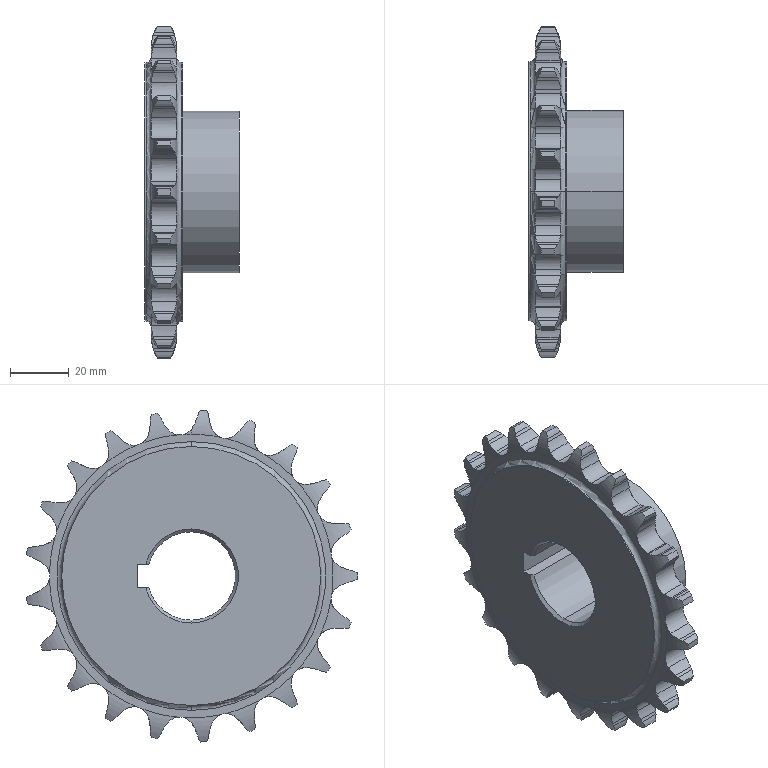Part | SolidWorks | features Chamfer 2, Cut 2, Revolution 2, CirPattern 1 | 1 solid | 249 faces | box 32 x 112.513 x 112.819 mm | volume 118760 mm3 | cylinder 145 | plane 50 | torus 48 | cone 6 | commonest cylinder face diameters 14.747 x44 26.567 x44 10.311 x27 113 x21 88 x4 30 x3